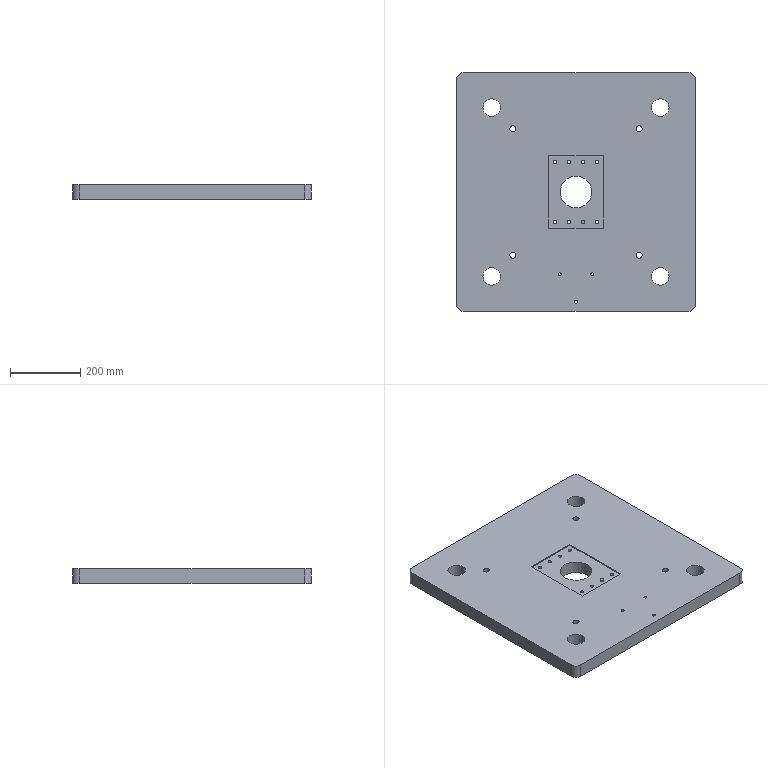Part | SolidWorks | features ICE 6, Extrusion 1, Fillet 1 | 1 solid | 56 faces | box 680 x 680 x 40 mm | volume 17772627 mm3 | cylinder 44 | plane 12 | commonest cylinder face diameters 10.1 x16 17.3 x8 50 x8 8.4 x6 40 x4 90 x2